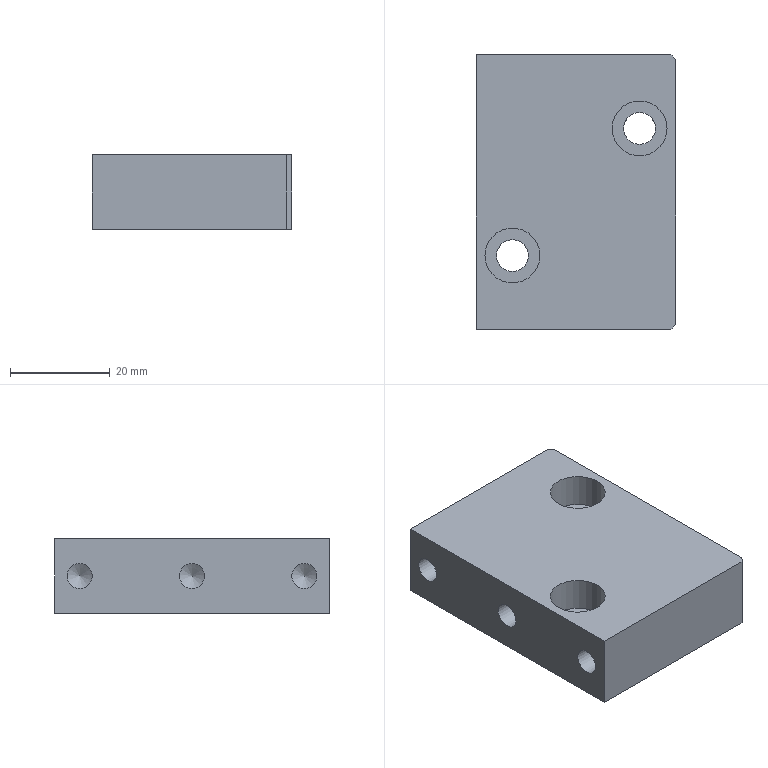Part | NX | 1 solid | 20 faces | box 40 x 55 x 15 mm | volume 30252 mm3 | plane 10 | cylinder 7 | cone 3 | commonest cylinder face diameters 5 x3 6.4 x2 11 x2
STEP:
#1=CARTESIAN_POINT('',(20.,-26.5,-7.5));
#2=VERTEX_POINT('',#1);
#3=CARTESIAN_POINT('',(20.,26.5,-7.5));
#4=VERTEX_POINT('',#3);
#5=CARTESIAN_POINT('',(20.,27.5,-7.5));
#6=DIRECTION('',(0.,1.,0.));
#7=VECTOR('',#6,1000.);
#8=LINE('',#5,#7);
#9=EDGE_CURVE('',#2,#4,#8,.T.);
#10=ORIENTED_EDGE('',*,*,#9,.T.);
#11=CARTESIAN_POINT('',(20.,26.5,7.5));
#12=VERTEX_POINT('',#11);
#13=CARTESIAN_POINT('',(20.,26.5,7.5));
#14=DIRECTION('',(0.,0.,1.));
#15=VECTOR('',#14,1000.);
#16=LINE('',#13,#15);
#17=EDGE_CURVE('',#4,#12,#16,.T.);
#18=ORIENTED_EDGE('',*,*,#17,.T.);
#19=CARTESIAN_POINT('',(20.,-26.5,7.5));
#20=VERTEX_POINT('',#19);
#21=CARTESIAN_POINT('',(20.,27.5,7.5));
#22=DIRECTION('',(0.,1.,0.));
#23=VECTOR('',#22,1000.);
#24=LINE('',#21,#23);
#25=EDGE_CURVE('',#20,#12,#24,.T.);
#26=ORIENTED_EDGE('',*,*,#25,.F.);
#27=CARTESIAN_POINT('',(20.,-26.5,7.5));
#28=DIRECTION('',(0.,0.,-1.));
#29=VECTOR('',#28,1000.);
#30=LINE('',#27,#29);
#31=EDGE_CURVE('',#20,#2,#30,.T.);
#32=ORIENTED_EDGE('',*,*,#31,.T.);
#33=EDGE_LOOP('',(#10,#18,#26,#32));
#34=FACE_BOUND('',#33,.T.);
#35=CARTESIAN_POINT('',(20.,27.5,7.5));
#36=DIRECTION('',(-1.,0.,0.));
#37=DIRECTION('',(0.,-1.,0.));
#38=AXIS2_PLACEMENT_3D('',#35,#36,#37);
#39=PLANE('',#38);
#40=ADVANCED_FACE('',(#34),#39,.F.);
#41=CARTESIAN_POINT('',(19.,27.5,7.5));
#42=VERTEX_POINT('',#41);
#43=CARTESIAN_POINT('',(-20.,27.5,7.5));
#44=VERTEX_POINT('',#43);
#45=CARTESIAN_POINT('',(-20.,27.5,7.5));
#46=DIRECTION('',(-1.,0.,0.));
#47=VECTOR('',#46,1000.);
#48=LINE('',#45,#47);
#49=EDGE_CURVE('',#42,#44,#48,.T.);
#50=ORIENTED_EDGE('',*,*,#49,.F.);
#51=CARTESIAN_POINT('',(19.,27.5,-7.5));
#52=VERTEX_POINT('',#51);
#53=CARTESIAN_POINT('',(19.,27.5,7.5));
#54=DIRECTION('',(0.,0.,-1.));
#55=VECTOR('',#54,1000.);
#56=LINE('',#53,#55);
#57=EDGE_CURVE('',#42,#52,#56,.T.);
#58=ORIENTED_EDGE('',*,*,#57,.T.);
#59=CARTESIAN_POINT('',(-20.,27.5,-7.5));
#60=VERTEX_POINT('',#59);
#61=CARTESIAN_POINT('',(-20.,27.5,-7.5));
#62=DIRECTION('',(-1.,0.,0.));
#63=VECTOR('',#62,1000.);
#64=LINE('',#61,#63);
#65=EDGE_CURVE('',#52,#60,#64,.T.);
#66=ORIENTED_EDGE('',*,*,#65,.T.);
#67=CARTESIAN_POINT('',(-20.,27.5,7.5));
#68=DIRECTION('',(0.,0.,-1.));
#69=VECTOR('',#68,1000.);
#70=LINE('',#67,#69);
#71=EDGE_CURVE('',#44,#60,#70,.T.);
#72=ORIENTED_EDGE('',*,*,#71,.F.);
#73=EDGE_LOOP('',(#50,#58,#66,#72));
#74=FACE_BOUND('',#73,.T.);
#75=CARTESIAN_POINT('',(-20.,27.5,7.5));
#76=DIRECTION('',(0.,-1.,0.));
#77=DIRECTION('',(0.,0.,-1.));
#78=AXIS2_PLACEMENT_3D('',#75,#76,#77);
#79=PLANE('',#78);
#80=ADVANCED_FACE('',(#74),#79,.F.);
#81=CARTESIAN_POINT('',(-20.,-22.5,2.5));
#82=VERTEX_POINT('',#81);
#83=CARTESIAN_POINT('',(-20.,-22.5,0.));
#84=DIRECTION('',(-1.,0.,0.));
#85=DIRECTION('',(0.,0.,1.));
#86=AXIS2_PLACEMENT_3D('',#83,#84,#85);
#87=CIRCLE('',#86,2.5);
#88=EDGE_CURVE('',#82,#82,#87,.T.);
#89=ORIENTED_EDGE('',*,*,#88,.F.);
#90=EDGE_LOOP('',(#89));
#91=FACE_BOUND('',#90,.T.);
#92=CARTESIAN_POINT('',(-20.,22.5,2.5));
#93=VERTEX_POINT('',#92);
#94=CARTESIAN_POINT('',(-20.,22.5,0.));
#95=DIRECTION('',(-1.,0.,0.));
#96=DIRECTION('',(0.,0.,1.));
#97=AXIS2_PLACEMENT_3D('',#94,#95,#96);
#98=CIRCLE('',#97,2.5);
#99=EDGE_CURVE('',#93,#93,#98,.T.);
#100=ORIENTED_EDGE('',*,*,#99,.F.);
#101=EDGE_LOOP('',(#100));
#102=FACE_BOUND('',#101,.T.);
#103=CARTESIAN_POINT('',(-20.,0.,2.5));
#104=VERTEX_POINT('',#103);
#105=CARTESIAN_POINT('',(-20.,0.,0.));
#106=DIRECTION('',(-1.,0.,0.));
#107=DIRECTION('',(0.,0.,1.));
#108=AXIS2_PLACEMENT_3D('',#105,#106,#107);
#109=CIRCLE('',#108,2.5);
#110=EDGE_CURVE('',#104,#104,#109,.T.);
#111=ORIENTED_EDGE('',*,*,#110,.F.);
#112=EDGE_LOOP('',(#111));
#113=FACE_BOUND('',#112,.T.);
#114=CARTESIAN_POINT('',(-20.,-27.5,-7.5));
#115=VERTEX_POINT('',#114);
#116=CARTESIAN_POINT('',(-20.,27.5,-7.5));
#117=DIRECTION('',(0.,-1.,0.));
#118=VECTOR('',#117,1000.);
#119=LINE('',#116,#118);
#120=EDGE_CURVE('',#60,#115,#119,.T.);
#121=ORIENTED_EDGE('',*,*,#120,.T.);
#122=CARTESIAN_POINT('',(-20.,-27.5,7.5));
#123=VERTEX_POINT('',#122);
#124=CARTESIAN_POINT('',(-20.,-27.5,7.5));
#125=DIRECTION('',(0.,0.,-1.));
#126=VECTOR('',#125,1000.);
#127=LINE('',#124,#126);
#128=EDGE_CURVE('',#123,#115,#127,.T.);
#129=ORIENTED_EDGE('',*,*,#128,.F.);
#130=CARTESIAN_POINT('',(-20.,27.5,7.5));
#131=DIRECTION('',(0.,-1.,0.));
#132=VECTOR('',#131,1000.);
#133=LINE('',#130,#132);
#134=EDGE_CURVE('',#44,#123,#133,.T.);
#135=ORIENTED_EDGE('',*,*,#134,.F.);
#136=ORIENTED_EDGE('',*,*,#71,.T.);
#137=EDGE_LOOP('',(#121,#129,#135,#136));
#138=FACE_BOUND('',#137,.T.);
#139=CARTESIAN_POINT('',(-20.,27.5,7.5));
#140=DIRECTION('',(1.,0.,0.));
#141=DIRECTION('',(0.,1.,0.));
#142=AXIS2_PLACEMENT_3D('',#139,#140,#141);
#143=PLANE('',#142);
#144=ADVANCED_FACE('',(#91,#102,#113,#138),#143,.F.);
#145=CARTESIAN_POINT('',(19.,-27.5,-7.5));
#146=VERTEX_POINT('',#145);
#147=CARTESIAN_POINT('',(-20.,-27.5,-7.5));
#148=DIRECTION('',(1.,0.,0.));
#149=VECTOR('',#148,1000.);
#150=LINE('',#147,#149);
#151=EDGE_CURVE('',#115,#146,#150,.T.);
#152=ORIENTED_EDGE('',*,*,#151,.T.);
#153=CARTESIAN_POINT('',(19.,-27.5,7.5));
#154=VERTEX_POINT('',#153);
#155=CARTESIAN_POINT('',(19.,-27.5,7.5));
#156=DIRECTION('',(0.,0.,1.));
#157=VECTOR('',#156,1000.);
#158=LINE('',#155,#157);
#159=EDGE_CURVE('',#146,#154,#158,.T.);
#160=ORIENTED_EDGE('',*,*,#159,.T.);
#161=CARTESIAN_POINT('',(-20.,-27.5,7.5));
#162=DIRECTION('',(1.,0.,0.));
#163=VECTOR('',#162,1000.);
#164=LINE('',#161,#163);
#165=EDGE_CURVE('',#123,#154,#164,.T.);
#166=ORIENTED_EDGE('',*,*,#165,.F.);
#167=ORIENTED_EDGE('',*,*,#128,.T.);
#168=EDGE_LOOP('',(#152,#160,#166,#167));
#169=FACE_BOUND('',#168,.T.);
#170=CARTESIAN_POINT('',(-20.,-27.5,7.5));
#171=DIRECTION('',(0.,1.,0.));
#172=DIRECTION('',(0.,0.,1.));
#173=AXIS2_PLACEMENT_3D('',#170,#171,#172);
#174=PLANE('',#173);
#175=ADVANCED_FACE('',(#169),#174,.F.);
#176=CARTESIAN_POINT('',(-7.228,-12.728,7.5));
#177=VERTEX_POINT('',#176);
#178=CARTESIAN_POINT('',(-12.728,-12.728,7.5));
#179=DIRECTION('',(0.,0.,1.));
#180=DIRECTION('',(1.,0.,0.));
#181=AXIS2_PLACEMENT_3D('',#178,#179,#180);
#182=CIRCLE('',#181,5.5);
#183=EDGE_CURVE('',#177,#177,#182,.T.);
#184=ORIENTED_EDGE('',*,*,#183,.F.);
#185=EDGE_LOOP('',(#184));
#186=FACE_BOUND('',#185,.T.);
#187=CARTESIAN_POINT('',(18.228,12.728,7.5));
#188=VERTEX_POINT('',#187);
#189=CARTESIAN_POINT('',(12.728,12.728,7.5));
#190=DIRECTION('',(0.,0.,1.));
#191=DIRECTION('',(1.,0.,0.));
#192=AXIS2_PLACEMENT_3D('',#189,#190,#191);
#193=CIRCLE('',#192,5.5);
#194=EDGE_CURVE('',#188,#188,#193,.T.);
#195=ORIENTED_EDGE('',*,*,#194,.F.);
#196=EDGE_LOOP('',(#195));
#197=FACE_BOUND('',#196,.T.);
#198=ORIENTED_EDGE('',*,*,#25,.T.);
#199=CARTESIAN_POINT('',(23.25,23.25,7.5));
#200=DIRECTION('',(0.7071,-0.7071,0.));
#201=VECTOR('',#200,1000.);
#202=LINE('',#199,#201);
#203=EDGE_CURVE('',#12,#42,#202,.F.);
#204=ORIENTED_EDGE('',*,*,#203,.T.);
#205=ORIENTED_EDGE('',*,*,#49,.T.);
#206=ORIENTED_EDGE('',*,*,#134,.T.);
#207=ORIENTED_EDGE('',*,*,#165,.T.);
#208=CARTESIAN_POINT('',(23.25,-23.25,7.5));
#209=DIRECTION('',(-0.7071,-0.7071,0.));
#210=VECTOR('',#209,1000.);
#211=LINE('',#208,#210);
#212=EDGE_CURVE('',#154,#20,#211,.F.);
#213=ORIENTED_EDGE('',*,*,#212,.T.);
#214=EDGE_LOOP('',(#198,#204,#205,#206,#207,#213));
#215=FACE_BOUND('',#214,.T.);
#216=CARTESIAN_POINT('',(0.,0.,7.5));
#217=DIRECTION('',(0.,0.,1.));
#218=DIRECTION('',(1.,0.,0.));
#219=AXIS2_PLACEMENT_3D('',#216,#217,#218);
#220=PLANE('',#219);
#221=ADVANCED_FACE('',(#186,#197,#215),#220,.T.);
#222=CARTESIAN_POINT('',(-9.528,-12.728,-7.5));
#223=VERTEX_POINT('',#222);
#224=CARTESIAN_POINT('',(-12.728,-12.728,-7.5));
#225=DIRECTION('',(0.,0.,1.));
#226=DIRECTION('',(1.,0.,0.));
#227=AXIS2_PLACEMENT_3D('',#224,#225,#226);
#228=CIRCLE('',#227,3.2);
#229=EDGE_CURVE('',#223,#223,#228,.T.);
#230=ORIENTED_EDGE('',*,*,#229,.T.);
#231=EDGE_LOOP('',(#230));
#232=FACE_BOUND('',#231,.T.);
#233=CARTESIAN_POINT('',(15.928,12.728,-7.5));
#234=VERTEX_POINT('',#233);
#235=CARTESIAN_POINT('',(12.728,12.728,-7.5));
#236=DIRECTION('',(0.,0.,1.));
#237=DIRECTION('',(1.,0.,0.));
#238=AXIS2_PLACEMENT_3D('',#235,#236,#237);
#239=CIRCLE('',#238,3.2);
#240=EDGE_CURVE('',#234,#234,#239,.T.);
#241=ORIENTED_EDGE('',*,*,#240,.T.);
#242=EDGE_LOOP('',(#241));
#243=FACE_BOUND('',#242,.T.);
#244=ORIENTED_EDGE('',*,*,#65,.F.);
#245=CARTESIAN_POINT('',(19.,27.5,-7.5));
#246=DIRECTION('',(-0.7071,0.7071,0.));
#247=VECTOR('',#246,1000.);
#248=LINE('',#245,#247);
#249=EDGE_CURVE('',#52,#4,#248,.F.);
#250=ORIENTED_EDGE('',*,*,#249,.T.);
#251=ORIENTED_EDGE('',*,*,#9,.F.);
#252=CARTESIAN_POINT('',(20.,-26.5,-7.5));
#253=DIRECTION('',(0.7071,0.7071,0.));
#254=VECTOR('',#253,1000.);
#255=LINE('',#252,#254);
#256=EDGE_CURVE('',#2,#146,#255,.F.);
#257=ORIENTED_EDGE('',*,*,#256,.T.);
#258=ORIENTED_EDGE('',*,*,#151,.F.);
#259=ORIENTED_EDGE('',*,*,#120,.F.);
#260=EDGE_LOOP('',(#244,#250,#251,#257,#258,#259));
#261=FACE_BOUND('',#260,.T.);
#262=CARTESIAN_POINT('',(0.,0.,-7.5));
#263=DIRECTION('',(0.,0.,1.));
#264=DIRECTION('',(1.,0.,0.));
#265=AXIS2_PLACEMENT_3D('',#262,#263,#264);
#266=PLANE('',#265);
#267=ADVANCED_FACE('',(#232,#243,#261),#266,.F.);
#268=ORIENTED_EDGE('',*,*,#203,.F.);
#269=ORIENTED_EDGE('',*,*,#17,.F.);
#270=ORIENTED_EDGE('',*,*,#249,.F.);
#271=ORIENTED_EDGE('',*,*,#57,.F.);
#272=EDGE_LOOP('',(#268,#269,#270,#271));
#273=FACE_BOUND('',#272,.T.);
#274=CARTESIAN_POINT('',(19.,27.5,7.5));
#275=DIRECTION('',(-0.7071,-0.7071,0.));
#276=DIRECTION('',(0.,0.,-1.));
#277=AXIS2_PLACEMENT_3D('',#274,#275,#276);
#278=PLANE('',#277);
#279=ADVANCED_FACE('',(#273),#278,.F.);
#280=ORIENTED_EDGE('',*,*,#212,.F.);
#281=ORIENTED_EDGE('',*,*,#159,.F.);
#282=ORIENTED_EDGE('',*,*,#256,.F.);
#283=ORIENTED_EDGE('',*,*,#31,.F.);
#284=EDGE_LOOP('',(#280,#281,#282,#283));
#285=FACE_BOUND('',#284,.T.);
#286=CARTESIAN_POINT('',(20.,-26.5,7.5));
#287=DIRECTION('',(-0.7071,0.7071,0.));
#288=DIRECTION('',(0.,0.,-1.));
#289=AXIS2_PLACEMENT_3D('',#286,#287,#288);
#290=PLANE('',#289);
#291=ADVANCED_FACE('',(#285),#290,.F.);
#292=CARTESIAN_POINT('',(-3.498,0.,0.));
#293=VERTEX_POINT('',#292);
#294=VERTEX_LOOP('',#293);
#295=FACE_BOUND('',#294,.T.);
#296=CARTESIAN_POINT('',(-5.,0.,2.5));
#297=VERTEX_POINT('',#296);
#298=CARTESIAN_POINT('',(-5.,0.,0.));
#299=DIRECTION('',(-1.,0.,0.));
#300=DIRECTION('',(0.,0.,1.));
#301=AXIS2_PLACEMENT_3D('',#298,#299,#300);
#302=CIRCLE('',#301,2.5);
#303=EDGE_CURVE('',#297,#297,#302,.T.);
#304=ORIENTED_EDGE('',*,*,#303,.T.);
#305=EDGE_LOOP('',(#304));
#306=FACE_BOUND('',#305,.T.);
#307=CARTESIAN_POINT('',(-5.,0.,0.));
#308=DIRECTION('',(-1.,0.,0.));
#309=DIRECTION('',(0.,0.,1.));
#310=AXIS2_PLACEMENT_3D('',#307,#308,#309);
#311=CONICAL_SURFACE('',#310,2.5,1.03);
#312=ADVANCED_FACE('',(#295,#306),#311,.F.);
#313=ORIENTED_EDGE('',*,*,#303,.F.);
#314=EDGE_LOOP('',(#313));
#315=FACE_BOUND('',#314,.T.);
#316=ORIENTED_EDGE('',*,*,#110,.T.);
#317=EDGE_LOOP('',(#316));
#318=FACE_BOUND('',#317,.T.);
#319=CARTESIAN_POINT('',(-20.,0.,0.));
#320=DIRECTION('',(-1.,0.,0.));
#321=DIRECTION('',(0.,0.,1.));
#322=AXIS2_PLACEMENT_3D('',#319,#320,#321);
#323=CYLINDRICAL_SURFACE('',#322,2.5);
#324=ADVANCED_FACE('',(#315,#318),#323,.F.);
#325=CARTESIAN_POINT('',(-3.498,22.5,0.));
#326=VERTEX_POINT('',#325);
#327=VERTEX_LOOP('',#326);
#328=FACE_BOUND('',#327,.T.);
#329=CARTESIAN_POINT('',(-5.,22.5,2.5));
#330=VERTEX_POINT('',#329);
#331=CARTESIAN_POINT('',(-5.,22.5,0.));
#332=DIRECTION('',(-1.,0.,0.));
#333=DIRECTION('',(0.,0.,1.));
#334=AXIS2_PLACEMENT_3D('',#331,#332,#333);
#335=CIRCLE('',#334,2.5);
#336=EDGE_CURVE('',#330,#330,#335,.T.);
#337=ORIENTED_EDGE('',*,*,#336,.T.);
#338=EDGE_LOOP('',(#337));
#339=FACE_BOUND('',#338,.T.);
#340=CARTESIAN_POINT('',(-5.,22.5,0.));
#341=DIRECTION('',(-1.,0.,0.));
#342=DIRECTION('',(0.,0.,1.));
#343=AXIS2_PLACEMENT_3D('',#340,#341,#342);
#344=CONICAL_SURFACE('',#343,2.5,1.03);
#345=ADVANCED_FACE('',(#328,#339),#344,.F.);
#346=ORIENTED_EDGE('',*,*,#336,.F.);
#347=EDGE_LOOP('',(#346));
#348=FACE_BOUND('',#347,.T.);
#349=ORIENTED_EDGE('',*,*,#99,.T.);
#350=EDGE_LOOP('',(#349));
#351=FACE_BOUND('',#350,.T.);
#352=CARTESIAN_POINT('',(-20.,22.5,0.));
#353=DIRECTION('',(-1.,0.,0.));
#354=DIRECTION('',(0.,0.,1.));
#355=AXIS2_PLACEMENT_3D('',#352,#353,#354);
#356=CYLINDRICAL_SURFACE('',#355,2.5);
#357=ADVANCED_FACE('',(#348,#351),#356,.F.);
#358=CARTESIAN_POINT('',(-3.498,-22.5,0.));
#359=VERTEX_POINT('',#358);
#360=VERTEX_LOOP('',#359);
#361=FACE_BOUND('',#360,.T.);
#362=CARTESIAN_POINT('',(-5.,-22.5,2.5));
#363=VERTEX_POINT('',#362);
#364=CARTESIAN_POINT('',(-5.,-22.5,0.));
#365=DIRECTION('',(-1.,0.,0.));
#366=DIRECTION('',(0.,0.,1.));
#367=AXIS2_PLACEMENT_3D('',#364,#365,#366);
#368=CIRCLE('',#367,2.5);
#369=EDGE_CURVE('',#363,#363,#368,.T.);
#370=ORIENTED_EDGE('',*,*,#369,.T.);
#371=EDGE_LOOP('',(#370));
#372=FACE_BOUND('',#371,.T.);
#373=CARTESIAN_POINT('',(-5.,-22.5,0.));
#374=DIRECTION('',(-1.,0.,0.));
#375=DIRECTION('',(0.,0.,1.));
#376=AXIS2_PLACEMENT_3D('',#373,#374,#375);
#377=CONICAL_SURFACE('',#376,2.5,1.03);
#378=ADVANCED_FACE('',(#361,#372),#377,.F.);
#379=ORIENTED_EDGE('',*,*,#369,.F.);
#380=EDGE_LOOP('',(#379));
#381=FACE_BOUND('',#380,.T.);
#382=ORIENTED_EDGE('',*,*,#88,.T.);
#383=EDGE_LOOP('',(#382));
#384=FACE_BOUND('',#383,.T.);
#385=CARTESIAN_POINT('',(-20.,-22.5,0.));
#386=DIRECTION('',(-1.,0.,0.));
#387=DIRECTION('',(0.,0.,1.));
#388=AXIS2_PLACEMENT_3D('',#385,#386,#387);
#389=CYLINDRICAL_SURFACE('',#388,2.5);
#390=ADVANCED_FACE('',(#381,#384),#389,.F.);
#391=ORIENTED_EDGE('',*,*,#240,.F.);
#392=EDGE_LOOP('',(#391));
#393=FACE_BOUND('',#392,.T.);
#394=CARTESIAN_POINT('',(15.928,12.728,0.7));
#395=VERTEX_POINT('',#394);
#396=CARTESIAN_POINT('',(12.728,12.728,0.7));
#397=DIRECTION('',(0.,0.,1.));
#398=DIRECTION('',(1.,0.,0.));
#399=AXIS2_PLACEMENT_3D('',#396,#397,#398);
#400=CIRCLE('',#399,3.2);
#401=EDGE_CURVE('',#395,#395,#400,.T.);
#402=ORIENTED_EDGE('',*,*,#401,.T.);
#403=EDGE_LOOP('',(#402));
#404=FACE_BOUND('',#403,.T.);
#405=CARTESIAN_POINT('',(12.728,12.728,7.5));
#406=DIRECTION('',(0.,0.,1.));
#407=DIRECTION('',(1.,0.,0.));
#408=AXIS2_PLACEMENT_3D('',#405,#406,#407);
#409=CYLINDRICAL_SURFACE('',#408,3.2);
#410=ADVANCED_FACE('',(#393,#404),#409,.F.);
#411=ORIENTED_EDGE('',*,*,#401,.F.);
#412=EDGE_LOOP('',(#411));
#413=FACE_BOUND('',#412,.T.);
#414=CARTESIAN_POINT('',(18.228,12.728,0.7));
#415=VERTEX_POINT('',#414);
#416=CARTESIAN_POINT('',(12.728,12.728,0.7));
#417=DIRECTION('',(0.,0.,1.));
#418=DIRECTION('',(1.,0.,0.));
#419=AXIS2_PLACEMENT_3D('',#416,#417,#418);
#420=CIRCLE('',#419,5.5);
#421=EDGE_CURVE('',#415,#415,#420,.T.);
#422=ORIENTED_EDGE('',*,*,#421,.T.);
#423=EDGE_LOOP('',(#422));
#424=FACE_BOUND('',#423,.T.);
#425=CARTESIAN_POINT('',(15.928,12.728,0.7));
#426=DIRECTION('',(0.,0.,-1.));
#427=DIRECTION('',(-1.,0.,0.));
#428=AXIS2_PLACEMENT_3D('',#425,#426,#427);
#429=PLANE('',#428);
#430=ADVANCED_FACE('',(#413,#424),#429,.F.);
#431=ORIENTED_EDGE('',*,*,#421,.F.);
#432=EDGE_LOOP('',(#431));
#433=FACE_BOUND('',#432,.T.);
#434=ORIENTED_EDGE('',*,*,#194,.T.);
#435=EDGE_LOOP('',(#434));
#436=FACE_BOUND('',#435,.T.);
#437=CARTESIAN_POINT('',(12.728,12.728,7.5));
#438=DIRECTION('',(0.,0.,1.));
#439=DIRECTION('',(1.,0.,0.));
#440=AXIS2_PLACEMENT_3D('',#437,#438,#439);
#441=CYLINDRICAL_SURFACE('',#440,5.5);
#442=ADVANCED_FACE('',(#433,#436),#441,.F.);
#443=ORIENTED_EDGE('',*,*,#229,.F.);
#444=EDGE_LOOP('',(#443));
#445=FACE_BOUND('',#444,.T.);
#446=CARTESIAN_POINT('',(-9.528,-12.728,0.7));
#447=VERTEX_POINT('',#446);
#448=CARTESIAN_POINT('',(-12.728,-12.728,0.7));
#449=DIRECTION('',(0.,0.,1.));
#450=DIRECTION('',(1.,0.,0.));
#451=AXIS2_PLACEMENT_3D('',#448,#449,#450);
#452=CIRCLE('',#451,3.2);
#453=EDGE_CURVE('',#447,#447,#452,.T.);
#454=ORIENTED_EDGE('',*,*,#453,.T.);
#455=EDGE_LOOP('',(#454));
#456=FACE_BOUND('',#455,.T.);
#457=CARTESIAN_POINT('',(-12.728,-12.728,7.5));
#458=DIRECTION('',(0.,0.,1.));
#459=DIRECTION('',(1.,0.,0.));
#460=AXIS2_PLACEMENT_3D('',#457,#458,#459);
#461=CYLINDRICAL_SURFACE('',#460,3.2);
#462=ADVANCED_FACE('',(#445,#456),#461,.F.);
#463=ORIENTED_EDGE('',*,*,#453,.F.);
#464=EDGE_LOOP('',(#463));
#465=FACE_BOUND('',#464,.T.);
#466=CARTESIAN_POINT('',(-7.228,-12.728,0.7));
#467=VERTEX_POINT('',#466);
#468=CARTESIAN_POINT('',(-12.728,-12.728,0.7));
#469=DIRECTION('',(0.,0.,1.));
#470=DIRECTION('',(1.,0.,0.));
#471=AXIS2_PLACEMENT_3D('',#468,#469,#470);
#472=CIRCLE('',#471,5.5);
#473=EDGE_CURVE('',#467,#467,#472,.T.);
#474=ORIENTED_EDGE('',*,*,#473,.T.);
#475=EDGE_LOOP('',(#474));
#476=FACE_BOUND('',#475,.T.);
#477=CARTESIAN_POINT('',(-9.528,-12.728,0.7));
#478=DIRECTION('',(0.,0.,-1.));
#479=DIRECTION('',(-1.,0.,0.));
#480=AXIS2_PLACEMENT_3D('',#477,#478,#479);
#481=PLANE('',#480);
#482=ADVANCED_FACE('',(#465,#476),#481,.F.);
#483=ORIENTED_EDGE('',*,*,#473,.F.);
#484=EDGE_LOOP('',(#483));
#485=FACE_BOUND('',#484,.T.);
#486=ORIENTED_EDGE('',*,*,#183,.T.);
#487=EDGE_LOOP('',(#486));
#488=FACE_BOUND('',#487,.T.);
#489=CARTESIAN_POINT('',(-12.728,-12.728,7.5));
#490=DIRECTION('',(0.,0.,1.));
#491=DIRECTION('',(1.,0.,0.));
#492=AXIS2_PLACEMENT_3D('',#489,#490,#491);
#493=CYLINDRICAL_SURFACE('',#492,5.5);
#494=ADVANCED_FACE('',(#485,#488),#493,.F.);
#495=CLOSED_SHELL('',(#40,#80,#144,#175,#221,#267,#279,#291,#312,#324,#345,#357,#378,#390,#410,#430,#442,#462,#482,#494));
#496=MANIFOLD_SOLID_BREP('',#495);
#497=(LENGTH_UNIT()NAMED_UNIT(*)SI_UNIT(.MILLI.,.METRE.));
#498=UNCERTAINTY_MEASURE_WITH_UNIT(LENGTH_MEASURE(0.00001),#497,'','');
#499=(NAMED_UNIT(*)PLANE_ANGLE_UNIT()SI_UNIT($,.RADIAN.));
#500=(NAMED_UNIT(*)SI_UNIT($,.STERADIAN.)SOLID_ANGLE_UNIT());
#501=(GEOMETRIC_REPRESENTATION_CONTEXT(3)GLOBAL_UNCERTAINTY_ASSIGNED_CONTEXT((#498))GLOBAL_UNIT_ASSIGNED_CONTEXT((#497,#499,#500))REPRESENTATION_CONTEXT('',''));
#502=ADVANCED_BREP_SHAPE_REPRESENTATION('',(#496),#501);